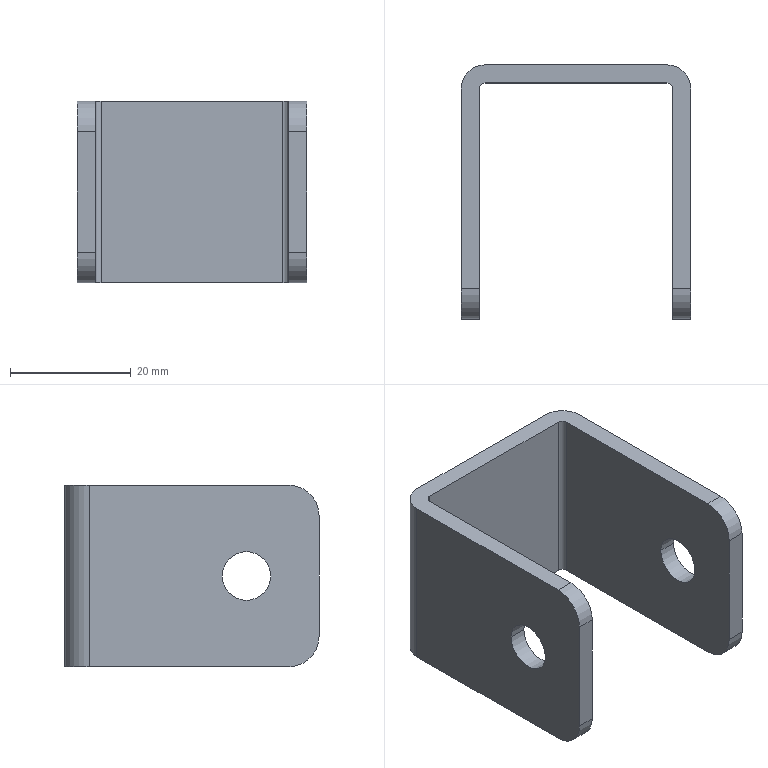Part | NX | features BLEND 1, DATUM_CSYS 1, EXTRACT_DATUM_PLANE 1, EXTRUDE 1, LINKED_BODY 1, SKETCH 1, SUBTRACT 1 | 1 solid | 22 faces | box 38 x 42 x 30 mm | volume 9881 mm3 | cylinder 12 | plane 10 | commonest cylinder face diameters 8 x6 10 x4 2 x2
STEP:
#1=CARTESIAN_POINT('',(-19.,-5.,0.));
#2=VERTEX_POINT('',#1);
#3=CARTESIAN_POINT('',(-19.,-13.,0.));
#4=VERTEX_POINT('',#3);
#5=CARTESIAN_POINT('',(-19.,-9.,0.));
#6=DIRECTION('',(-1.,0.,0.));
#7=DIRECTION('',(0.,0.,1.));
#8=AXIS2_PLACEMENT_3D('',#5,#6,#7);
#9=CIRCLE('',#8,4.);
#10=EDGE_CURVE('',#2,#4,#9,.T.);
#11=ORIENTED_EDGE('',*,*,#10,.F.);
#12=CARTESIAN_POINT('',(-19.,-9.,0.));
#13=DIRECTION('',(-1.,0.,0.));
#14=DIRECTION('',(0.,0.,1.));
#15=AXIS2_PLACEMENT_3D('',#12,#13,#14);
#16=CIRCLE('',#15,4.);
#17=EDGE_CURVE('',#4,#2,#16,.T.);
#18=ORIENTED_EDGE('',*,*,#17,.F.);
#19=EDGE_LOOP('',(#11,#18));
#20=FACE_BOUND('',#19,.T.);
#21=CARTESIAN_POINT('',(-19.,-21.,10.));
#22=VERTEX_POINT('',#21);
#23=CARTESIAN_POINT('',(-19.,-21.,-10.));
#24=VERTEX_POINT('',#23);
#25=CARTESIAN_POINT('',(-19.,-21.,15.));
#26=DIRECTION('',(0.,0.,-1.));
#27=VECTOR('',#26,1000.);
#28=LINE('',#25,#27);
#29=EDGE_CURVE('',#22,#24,#28,.T.);
#30=ORIENTED_EDGE('',*,*,#29,.F.);
#31=CARTESIAN_POINT('',(-19.,-16.,15.));
#32=VERTEX_POINT('',#31);
#33=CARTESIAN_POINT('',(-19.,-16.,10.));
#34=DIRECTION('',(-1.,0.,0.));
#35=DIRECTION('',(0.,0.,1.));
#36=AXIS2_PLACEMENT_3D('',#33,#34,#35);
#37=CIRCLE('',#36,5.);
#38=EDGE_CURVE('',#22,#32,#37,.T.);
#39=ORIENTED_EDGE('',*,*,#38,.T.);
#40=CARTESIAN_POINT('',(-19.,17.,15.));
#41=VERTEX_POINT('',#40);
#42=CARTESIAN_POINT('',(-19.,-21.,15.));
#43=DIRECTION('',(0.,1.,0.));
#44=VECTOR('',#43,1000.);
#45=LINE('',#42,#44);
#46=EDGE_CURVE('',#41,#32,#45,.F.);
#47=ORIENTED_EDGE('',*,*,#46,.F.);
#48=CARTESIAN_POINT('',(-19.,17.,-15.));
#49=VERTEX_POINT('',#48);
#50=CARTESIAN_POINT('',(-19.,17.,15.));
#51=DIRECTION('',(0.,0.,-1.));
#52=VECTOR('',#51,1000.);
#53=LINE('',#50,#52);
#54=EDGE_CURVE('',#41,#49,#53,.T.);
#55=ORIENTED_EDGE('',*,*,#54,.T.);
#56=CARTESIAN_POINT('',(-19.,-16.,-15.));
#57=VERTEX_POINT('',#56);
#58=CARTESIAN_POINT('',(-19.,-16.,-15.));
#59=DIRECTION('',(0.,1.,0.));
#60=VECTOR('',#59,1000.);
#61=LINE('',#58,#60);
#62=EDGE_CURVE('',#57,#49,#61,.T.);
#63=ORIENTED_EDGE('',*,*,#62,.F.);
#64=CARTESIAN_POINT('',(-19.,-16.,-10.));
#65=DIRECTION('',(-1.,0.,0.));
#66=DIRECTION('',(0.,0.,1.));
#67=AXIS2_PLACEMENT_3D('',#64,#65,#66);
#68=CIRCLE('',#67,5.);
#69=EDGE_CURVE('',#57,#24,#68,.T.);
#70=ORIENTED_EDGE('',*,*,#69,.T.);
#71=EDGE_LOOP('',(#30,#39,#47,#55,#63,#70));
#72=FACE_BOUND('',#71,.T.);
#73=CARTESIAN_POINT('',(-19.,-16.,15.));
#74=DIRECTION('',(-1.,0.,0.));
#75=DIRECTION('',(0.,0.,1.));
#76=AXIS2_PLACEMENT_3D('',#73,#74,#75);
#77=PLANE('',#76);
#78=ADVANCED_FACE('',(#20,#72),#77,.T.);
#79=CARTESIAN_POINT('',(-15.,21.,-15.));
#80=VERTEX_POINT('',#79);
#81=CARTESIAN_POINT('',(-15.,17.,-15.));
#82=DIRECTION('',(0.,0.,-1.));
#83=DIRECTION('',(-1.,0.,0.));
#84=AXIS2_PLACEMENT_3D('',#81,#82,#83);
#85=CIRCLE('',#84,4.);
#86=EDGE_CURVE('',#49,#80,#85,.T.);
#87=ORIENTED_EDGE('',*,*,#86,.F.);
#88=ORIENTED_EDGE('',*,*,#54,.F.);
#89=CARTESIAN_POINT('',(-15.,21.,15.));
#90=VERTEX_POINT('',#89);
#91=CARTESIAN_POINT('',(-15.,17.,15.));
#92=DIRECTION('',(0.,0.,-1.));
#93=DIRECTION('',(-1.,0.,0.));
#94=AXIS2_PLACEMENT_3D('',#91,#92,#93);
#95=CIRCLE('',#94,4.);
#96=EDGE_CURVE('',#90,#41,#95,.F.);
#97=ORIENTED_EDGE('',*,*,#96,.F.);
#98=CARTESIAN_POINT('',(-15.,21.,15.));
#99=DIRECTION('',(0.,0.,-1.));
#100=VECTOR('',#99,1000.);
#101=LINE('',#98,#100);
#102=EDGE_CURVE('',#90,#80,#101,.T.);
#103=ORIENTED_EDGE('',*,*,#102,.T.);
#104=EDGE_LOOP('',(#87,#88,#97,#103));
#105=FACE_BOUND('',#104,.T.);
#106=CARTESIAN_POINT('',(-15.,17.,15.));
#107=DIRECTION('',(0.,0.,-1.));
#108=DIRECTION('',(-1.,0.,0.));
#109=AXIS2_PLACEMENT_3D('',#106,#107,#108);
#110=CYLINDRICAL_SURFACE('',#109,4.);
#111=ADVANCED_FACE('',(#105),#110,.T.);
#112=CARTESIAN_POINT('',(15.,21.,-15.));
#113=VERTEX_POINT('',#112);
#114=CARTESIAN_POINT('',(-15.,21.,-15.));
#115=DIRECTION('',(1.,0.,0.));
#116=VECTOR('',#115,1000.);
#117=LINE('',#114,#116);
#118=EDGE_CURVE('',#80,#113,#117,.T.);
#119=ORIENTED_EDGE('',*,*,#118,.F.);
#120=ORIENTED_EDGE('',*,*,#102,.F.);
#121=CARTESIAN_POINT('',(15.,21.,15.));
#122=VERTEX_POINT('',#121);
#123=CARTESIAN_POINT('',(-15.,21.,15.));
#124=DIRECTION('',(1.,0.,0.));
#125=VECTOR('',#124,1000.);
#126=LINE('',#123,#125);
#127=EDGE_CURVE('',#122,#90,#126,.F.);
#128=ORIENTED_EDGE('',*,*,#127,.F.);
#129=CARTESIAN_POINT('',(15.,21.,15.));
#130=DIRECTION('',(0.,0.,-1.));
#131=VECTOR('',#130,1000.);
#132=LINE('',#129,#131);
#133=EDGE_CURVE('',#122,#113,#132,.T.);
#134=ORIENTED_EDGE('',*,*,#133,.T.);
#135=EDGE_LOOP('',(#119,#120,#128,#134));
#136=FACE_BOUND('',#135,.T.);
#137=CARTESIAN_POINT('',(-15.,21.,15.));
#138=DIRECTION('',(0.,1.,0.));
#139=DIRECTION('',(0.,0.,1.));
#140=AXIS2_PLACEMENT_3D('',#137,#138,#139);
#141=PLANE('',#140);
#142=ADVANCED_FACE('',(#136),#141,.T.);
#143=CARTESIAN_POINT('',(19.,17.,-15.));
#144=VERTEX_POINT('',#143);
#145=CARTESIAN_POINT('',(15.,17.,-15.));
#146=DIRECTION('',(0.,0.,-1.));
#147=DIRECTION('',(0.,1.,0.));
#148=AXIS2_PLACEMENT_3D('',#145,#146,#147);
#149=CIRCLE('',#148,4.);
#150=EDGE_CURVE('',#113,#144,#149,.T.);
#151=ORIENTED_EDGE('',*,*,#150,.F.);
#152=ORIENTED_EDGE('',*,*,#133,.F.);
#153=CARTESIAN_POINT('',(19.,17.,15.));
#154=VERTEX_POINT('',#153);
#155=CARTESIAN_POINT('',(15.,17.,15.));
#156=DIRECTION('',(0.,0.,-1.));
#157=DIRECTION('',(0.,1.,0.));
#158=AXIS2_PLACEMENT_3D('',#155,#156,#157);
#159=CIRCLE('',#158,4.);
#160=EDGE_CURVE('',#154,#122,#159,.F.);
#161=ORIENTED_EDGE('',*,*,#160,.F.);
#162=CARTESIAN_POINT('',(19.,17.,15.));
#163=DIRECTION('',(0.,0.,-1.));
#164=VECTOR('',#163,1000.);
#165=LINE('',#162,#164);
#166=EDGE_CURVE('',#154,#144,#165,.T.);
#167=ORIENTED_EDGE('',*,*,#166,.T.);
#168=EDGE_LOOP('',(#151,#152,#161,#167));
#169=FACE_BOUND('',#168,.T.);
#170=CARTESIAN_POINT('',(15.,17.,15.));
#171=DIRECTION('',(0.,0.,-1.));
#172=DIRECTION('',(-1.,0.,0.));
#173=AXIS2_PLACEMENT_3D('',#170,#171,#172);
#174=CYLINDRICAL_SURFACE('',#173,4.);
#175=ADVANCED_FACE('',(#169),#174,.T.);
#176=CARTESIAN_POINT('',(19.,-16.,15.));
#177=VERTEX_POINT('',#176);
#178=CARTESIAN_POINT('',(19.,17.,15.));
#179=DIRECTION('',(0.,-1.,0.));
#180=VECTOR('',#179,1000.);
#181=LINE('',#178,#180);
#182=EDGE_CURVE('',#177,#154,#181,.F.);
#183=ORIENTED_EDGE('',*,*,#182,.F.);
#184=CARTESIAN_POINT('',(19.,-21.,10.));
#185=VERTEX_POINT('',#184);
#186=CARTESIAN_POINT('',(19.,-16.,10.));
#187=DIRECTION('',(1.,0.,0.));
#188=DIRECTION('',(0.,0.,-1.));
#189=AXIS2_PLACEMENT_3D('',#186,#187,#188);
#190=CIRCLE('',#189,5.);
#191=EDGE_CURVE('',#177,#185,#190,.T.);
#192=ORIENTED_EDGE('',*,*,#191,.T.);
#193=CARTESIAN_POINT('',(19.,-21.,-10.));
#194=VERTEX_POINT('',#193);
#195=CARTESIAN_POINT('',(19.,-21.,15.));
#196=DIRECTION('',(0.,0.,-1.));
#197=VECTOR('',#196,1000.);
#198=LINE('',#195,#197);
#199=EDGE_CURVE('',#185,#194,#198,.T.);
#200=ORIENTED_EDGE('',*,*,#199,.T.);
#201=CARTESIAN_POINT('',(19.,-16.,-15.));
#202=VERTEX_POINT('',#201);
#203=CARTESIAN_POINT('',(19.,-16.,-10.));
#204=DIRECTION('',(1.,0.,0.));
#205=DIRECTION('',(0.,0.,-1.));
#206=AXIS2_PLACEMENT_3D('',#203,#204,#205);
#207=CIRCLE('',#206,5.);
#208=EDGE_CURVE('',#194,#202,#207,.T.);
#209=ORIENTED_EDGE('',*,*,#208,.T.);
#210=CARTESIAN_POINT('',(19.,-16.,-15.));
#211=DIRECTION('',(0.,-1.,0.));
#212=VECTOR('',#211,1000.);
#213=LINE('',#210,#212);
#214=EDGE_CURVE('',#144,#202,#213,.T.);
#215=ORIENTED_EDGE('',*,*,#214,.F.);
#216=ORIENTED_EDGE('',*,*,#166,.F.);
#217=EDGE_LOOP('',(#183,#192,#200,#209,#215,#216));
#218=FACE_BOUND('',#217,.T.);
#219=CARTESIAN_POINT('',(19.,-13.,0.));
#220=VERTEX_POINT('',#219);
#221=CARTESIAN_POINT('',(19.,-5.,0.));
#222=VERTEX_POINT('',#221);
#223=CARTESIAN_POINT('',(19.,-9.,0.));
#224=DIRECTION('',(1.,0.,0.));
#225=DIRECTION('',(0.,-1.,0.));
#226=AXIS2_PLACEMENT_3D('',#223,#224,#225);
#227=CIRCLE('',#226,4.);
#228=EDGE_CURVE('',#220,#222,#227,.T.);
#229=ORIENTED_EDGE('',*,*,#228,.F.);
#230=CARTESIAN_POINT('',(19.,-9.,0.));
#231=DIRECTION('',(1.,0.,0.));
#232=DIRECTION('',(0.,1.,0.));
#233=AXIS2_PLACEMENT_3D('',#230,#231,#232);
#234=CIRCLE('',#233,4.);
#235=EDGE_CURVE('',#222,#220,#234,.T.);
#236=ORIENTED_EDGE('',*,*,#235,.F.);
#237=EDGE_LOOP('',(#229,#236));
#238=FACE_BOUND('',#237,.T.);
#239=CARTESIAN_POINT('',(19.,-16.,15.));
#240=DIRECTION('',(1.,0.,0.));
#241=DIRECTION('',(0.,0.,-1.));
#242=AXIS2_PLACEMENT_3D('',#239,#240,#241);
#243=PLANE('',#242);
#244=ADVANCED_FACE('',(#218,#238),#243,.T.);
#245=ORIENTED_EDGE('',*,*,#199,.F.);
#246=CARTESIAN_POINT('',(16.,-21.,10.));
#247=VERTEX_POINT('',#246);
#248=CARTESIAN_POINT('',(16.,-21.,10.));
#249=DIRECTION('',(1.,0.,0.));
#250=VECTOR('',#249,1000.);
#251=LINE('',#248,#250);
#252=EDGE_CURVE('',#185,#247,#251,.F.);
#253=ORIENTED_EDGE('',*,*,#252,.T.);
#254=CARTESIAN_POINT('',(16.,-21.,-10.));
#255=VERTEX_POINT('',#254);
#256=CARTESIAN_POINT('',(16.,-21.,15.));
#257=DIRECTION('',(0.,0.,-1.));
#258=VECTOR('',#257,1000.);
#259=LINE('',#256,#258);
#260=EDGE_CURVE('',#247,#255,#259,.T.);
#261=ORIENTED_EDGE('',*,*,#260,.T.);
#262=CARTESIAN_POINT('',(19.,-21.,-10.));
#263=DIRECTION('',(-1.,0.,0.));
#264=VECTOR('',#263,1000.);
#265=LINE('',#262,#264);
#266=EDGE_CURVE('',#255,#194,#265,.F.);
#267=ORIENTED_EDGE('',*,*,#266,.T.);
#268=EDGE_LOOP('',(#245,#253,#261,#267));
#269=FACE_BOUND('',#268,.T.);
#270=CARTESIAN_POINT('',(19.,-21.,15.));
#271=DIRECTION('',(0.,-1.,0.));
#272=DIRECTION('',(0.,0.,-1.));
#273=AXIS2_PLACEMENT_3D('',#270,#271,#272);
#274=PLANE('',#273);
#275=ADVANCED_FACE('',(#269),#274,.T.);
#276=CARTESIAN_POINT('',(16.,-5.,0.));
#277=VERTEX_POINT('',#276);
#278=CARTESIAN_POINT('',(16.,-13.,0.));
#279=VERTEX_POINT('',#278);
#280=CARTESIAN_POINT('',(16.,-9.,0.));
#281=DIRECTION('',(-1.,0.,0.));
#282=DIRECTION('',(0.,0.,1.));
#283=AXIS2_PLACEMENT_3D('',#280,#281,#282);
#284=CIRCLE('',#283,4.);
#285=EDGE_CURVE('',#277,#279,#284,.T.);
#286=ORIENTED_EDGE('',*,*,#285,.F.);
#287=CARTESIAN_POINT('',(16.,-9.,0.));
#288=DIRECTION('',(-1.,0.,0.));
#289=DIRECTION('',(0.,0.,1.));
#290=AXIS2_PLACEMENT_3D('',#287,#288,#289);
#291=CIRCLE('',#290,4.);
#292=EDGE_CURVE('',#279,#277,#291,.T.);
#293=ORIENTED_EDGE('',*,*,#292,.F.);
#294=EDGE_LOOP('',(#286,#293));
#295=FACE_BOUND('',#294,.T.);
#296=ORIENTED_EDGE('',*,*,#260,.F.);
#297=CARTESIAN_POINT('',(16.,-16.,15.));
#298=VERTEX_POINT('',#297);
#299=CARTESIAN_POINT('',(16.,-16.,10.));
#300=DIRECTION('',(-1.,0.,0.));
#301=DIRECTION('',(0.,0.,1.));
#302=AXIS2_PLACEMENT_3D('',#299,#300,#301);
#303=CIRCLE('',#302,5.);
#304=EDGE_CURVE('',#247,#298,#303,.T.);
#305=ORIENTED_EDGE('',*,*,#304,.T.);
#306=CARTESIAN_POINT('',(16.,17.,15.));
#307=VERTEX_POINT('',#306);
#308=CARTESIAN_POINT('',(16.,-21.,15.));
#309=DIRECTION('',(0.,1.,0.));
#310=VECTOR('',#309,1000.);
#311=LINE('',#308,#310);
#312=EDGE_CURVE('',#307,#298,#311,.F.);
#313=ORIENTED_EDGE('',*,*,#312,.F.);
#314=CARTESIAN_POINT('',(16.,17.,-15.));
#315=VERTEX_POINT('',#314);
#316=CARTESIAN_POINT('',(16.,17.,15.));
#317=DIRECTION('',(0.,0.,-1.));
#318=VECTOR('',#317,1000.);
#319=LINE('',#316,#318);
#320=EDGE_CURVE('',#307,#315,#319,.T.);
#321=ORIENTED_EDGE('',*,*,#320,.T.);
#322=CARTESIAN_POINT('',(16.,-16.,-15.));
#323=VERTEX_POINT('',#322);
#324=CARTESIAN_POINT('',(16.,-16.,-15.));
#325=DIRECTION('',(0.,1.,0.));
#326=VECTOR('',#325,1000.);
#327=LINE('',#324,#326);
#328=EDGE_CURVE('',#323,#315,#327,.T.);
#329=ORIENTED_EDGE('',*,*,#328,.F.);
#330=CARTESIAN_POINT('',(16.,-16.,-10.));
#331=DIRECTION('',(-1.,0.,0.));
#332=DIRECTION('',(0.,0.,1.));
#333=AXIS2_PLACEMENT_3D('',#330,#331,#332);
#334=CIRCLE('',#333,5.);
#335=EDGE_CURVE('',#323,#255,#334,.T.);
#336=ORIENTED_EDGE('',*,*,#335,.T.);
#337=EDGE_LOOP('',(#296,#305,#313,#321,#329,#336));
#338=FACE_BOUND('',#337,.T.);
#339=CARTESIAN_POINT('',(16.,-16.,15.));
#340=DIRECTION('',(-1.,0.,0.));
#341=DIRECTION('',(0.,0.,1.));
#342=AXIS2_PLACEMENT_3D('',#339,#340,#341);
#343=PLANE('',#342);
#344=ADVANCED_FACE('',(#295,#338),#343,.T.);
#345=CARTESIAN_POINT('',(15.,18.,-15.));
#346=VERTEX_POINT('',#345);
#347=CARTESIAN_POINT('',(15.,17.,-15.));
#348=DIRECTION('',(0.,0.,1.));
#349=DIRECTION('',(1.,0.,0.));
#350=AXIS2_PLACEMENT_3D('',#347,#348,#349);
#351=CIRCLE('',#350,1.);
#352=EDGE_CURVE('',#315,#346,#351,.T.);
#353=ORIENTED_EDGE('',*,*,#352,.F.);
#354=ORIENTED_EDGE('',*,*,#320,.F.);
#355=CARTESIAN_POINT('',(15.,18.,15.));
#356=VERTEX_POINT('',#355);
#357=CARTESIAN_POINT('',(15.,17.,15.));
#358=DIRECTION('',(0.,0.,1.));
#359=DIRECTION('',(1.,0.,0.));
#360=AXIS2_PLACEMENT_3D('',#357,#358,#359);
#361=CIRCLE('',#360,1.);
#362=EDGE_CURVE('',#356,#307,#361,.F.);
#363=ORIENTED_EDGE('',*,*,#362,.F.);
#364=CARTESIAN_POINT('',(15.,18.,15.));
#365=DIRECTION('',(0.,0.,-1.));
#366=VECTOR('',#365,1000.);
#367=LINE('',#364,#366);
#368=EDGE_CURVE('',#356,#346,#367,.T.);
#369=ORIENTED_EDGE('',*,*,#368,.T.);
#370=EDGE_LOOP('',(#353,#354,#363,#369));
#371=FACE_BOUND('',#370,.T.);
#372=CARTESIAN_POINT('',(15.,17.,15.));
#373=DIRECTION('',(0.,0.,-1.));
#374=DIRECTION('',(-1.,0.,0.));
#375=AXIS2_PLACEMENT_3D('',#372,#373,#374);
#376=CYLINDRICAL_SURFACE('',#375,1.);
#377=ADVANCED_FACE('',(#371),#376,.F.);
#378=CARTESIAN_POINT('',(-15.,18.,-15.));
#379=VERTEX_POINT('',#378);
#380=CARTESIAN_POINT('',(15.,18.,-15.));
#381=DIRECTION('',(-1.,0.,0.));
#382=VECTOR('',#381,1000.);
#383=LINE('',#380,#382);
#384=EDGE_CURVE('',#346,#379,#383,.T.);
#385=ORIENTED_EDGE('',*,*,#384,.F.);
#386=ORIENTED_EDGE('',*,*,#368,.F.);
#387=CARTESIAN_POINT('',(-15.,18.,15.));
#388=VERTEX_POINT('',#387);
#389=CARTESIAN_POINT('',(15.,18.,15.));
#390=DIRECTION('',(-1.,0.,0.));
#391=VECTOR('',#390,1000.);
#392=LINE('',#389,#391);
#393=EDGE_CURVE('',#388,#356,#392,.F.);
#394=ORIENTED_EDGE('',*,*,#393,.F.);
#395=CARTESIAN_POINT('',(-15.,18.,15.));
#396=DIRECTION('',(0.,0.,-1.));
#397=VECTOR('',#396,1000.);
#398=LINE('',#395,#397);
#399=EDGE_CURVE('',#388,#379,#398,.T.);
#400=ORIENTED_EDGE('',*,*,#399,.T.);
#401=EDGE_LOOP('',(#385,#386,#394,#400));
#402=FACE_BOUND('',#401,.T.);
#403=CARTESIAN_POINT('',(15.,18.,15.));
#404=DIRECTION('',(0.,-1.,0.));
#405=DIRECTION('',(0.,0.,-1.));
#406=AXIS2_PLACEMENT_3D('',#403,#404,#405);
#407=PLANE('',#406);
#408=ADVANCED_FACE('',(#402),#407,.T.);
#409=CARTESIAN_POINT('',(-16.,17.,-15.));
#410=VERTEX_POINT('',#409);
#411=CARTESIAN_POINT('',(-15.,17.,-15.));
#412=DIRECTION('',(0.,0.,1.));
#413=DIRECTION('',(0.,1.,0.));
#414=AXIS2_PLACEMENT_3D('',#411,#412,#413);
#415=CIRCLE('',#414,1.);
#416=EDGE_CURVE('',#379,#410,#415,.T.);
#417=ORIENTED_EDGE('',*,*,#416,.F.);
#418=ORIENTED_EDGE('',*,*,#399,.F.);
#419=CARTESIAN_POINT('',(-16.,17.,15.));
#420=VERTEX_POINT('',#419);
#421=CARTESIAN_POINT('',(-15.,17.,15.));
#422=DIRECTION('',(0.,0.,1.));
#423=DIRECTION('',(0.,1.,0.));
#424=AXIS2_PLACEMENT_3D('',#421,#422,#423);
#425=CIRCLE('',#424,1.);
#426=EDGE_CURVE('',#420,#388,#425,.F.);
#427=ORIENTED_EDGE('',*,*,#426,.F.);
#428=CARTESIAN_POINT('',(-16.,17.,15.));
#429=DIRECTION('',(0.,0.,-1.));
#430=VECTOR('',#429,1000.);
#431=LINE('',#428,#430);
#432=EDGE_CURVE('',#420,#410,#431,.T.);
#433=ORIENTED_EDGE('',*,*,#432,.T.);
#434=EDGE_LOOP('',(#417,#418,#427,#433));
#435=FACE_BOUND('',#434,.T.);
#436=CARTESIAN_POINT('',(-15.,17.,15.));
#437=DIRECTION('',(0.,0.,-1.));
#438=DIRECTION('',(-1.,0.,0.));
#439=AXIS2_PLACEMENT_3D('',#436,#437,#438);
#440=CYLINDRICAL_SURFACE('',#439,1.);
#441=ADVANCED_FACE('',(#435),#440,.F.);
#442=CARTESIAN_POINT('',(-16.,-13.,0.));
#443=VERTEX_POINT('',#442);
#444=CARTESIAN_POINT('',(-16.,-5.,0.));
#445=VERTEX_POINT('',#444);
#446=CARTESIAN_POINT('',(-16.,-9.,0.));
#447=DIRECTION('',(1.,0.,0.));
#448=DIRECTION('',(0.,0.,-1.));
#449=AXIS2_PLACEMENT_3D('',#446,#447,#448);
#450=CIRCLE('',#449,4.);
#451=EDGE_CURVE('',#443,#445,#450,.T.);
#452=ORIENTED_EDGE('',*,*,#451,.F.);
#453=CARTESIAN_POINT('',(-16.,-9.,0.));
#454=DIRECTION('',(1.,0.,0.));
#455=DIRECTION('',(0.,0.,-1.));
#456=AXIS2_PLACEMENT_3D('',#453,#454,#455);
#457=CIRCLE('',#456,4.);
#458=EDGE_CURVE('',#445,#443,#457,.T.);
#459=ORIENTED_EDGE('',*,*,#458,.F.);
#460=EDGE_LOOP('',(#452,#459));
#461=FACE_BOUND('',#460,.T.);
#462=CARTESIAN_POINT('',(-16.,-16.,15.));
#463=VERTEX_POINT('',#462);
#464=CARTESIAN_POINT('',(-16.,17.,15.));
#465=DIRECTION('',(0.,-1.,0.));
#466=VECTOR('',#465,1000.);
#467=LINE('',#464,#466);
#468=EDGE_CURVE('',#463,#420,#467,.F.);
#469=ORIENTED_EDGE('',*,*,#468,.F.);
#470=CARTESIAN_POINT('',(-16.,-21.,10.));
#471=VERTEX_POINT('',#470);
#472=CARTESIAN_POINT('',(-16.,-16.,10.));
#473=DIRECTION('',(1.,0.,0.));
#474=DIRECTION('',(0.,0.,-1.));
#475=AXIS2_PLACEMENT_3D('',#472,#473,#474);
#476=CIRCLE('',#475,5.);
#477=EDGE_CURVE('',#463,#471,#476,.T.);
#478=ORIENTED_EDGE('',*,*,#477,.T.);
#479=CARTESIAN_POINT('',(-16.,-21.,-10.));
#480=VERTEX_POINT('',#479);
#481=CARTESIAN_POINT('',(-16.,-21.,15.));
#482=DIRECTION('',(0.,0.,-1.));
#483=VECTOR('',#482,1000.);
#484=LINE('',#481,#483);
#485=EDGE_CURVE('',#471,#480,#484,.T.);
#486=ORIENTED_EDGE('',*,*,#485,.T.);
#487=CARTESIAN_POINT('',(-16.,-16.,-15.));
#488=VERTEX_POINT('',#487);
#489=CARTESIAN_POINT('',(-16.,-16.,-10.));
#490=DIRECTION('',(1.,0.,0.));
#491=DIRECTION('',(0.,0.,-1.));
#492=AXIS2_PLACEMENT_3D('',#489,#490,#491);
#493=CIRCLE('',#492,5.);
#494=EDGE_CURVE('',#480,#488,#493,.T.);
#495=ORIENTED_EDGE('',*,*,#494,.T.);
#496=CARTESIAN_POINT('',(-16.,-16.,-15.));
#497=DIRECTION('',(0.,-1.,0.));
#498=VECTOR('',#497,1000.);
#499=LINE('',#496,#498);
#500=EDGE_CURVE('',#410,#488,#499,.T.);
#501=ORIENTED_EDGE('',*,*,#500,.F.);
#502=ORIENTED_EDGE('',*,*,#432,.F.);
#503=EDGE_LOOP('',(#469,#478,#486,#495,#501,#502));
#504=FACE_BOUND('',#503,.T.);
#505=CARTESIAN_POINT('',(-16.,-16.,15.));
#506=DIRECTION('',(1.,0.,0.));
#507=DIRECTION('',(0.,0.,-1.));
#508=AXIS2_PLACEMENT_3D('',#505,#506,#507);
#509=PLANE('',#508);
#510=ADVANCED_FACE('',(#461,#504),#509,.T.);
#511=ORIENTED_EDGE('',*,*,#485,.F.);
#512=CARTESIAN_POINT('',(-19.,-21.,10.));
#513=DIRECTION('',(1.,0.,0.));
#514=VECTOR('',#513,1000.);
#515=LINE('',#512,#514);
#516=EDGE_CURVE('',#471,#22,#515,.F.);
#517=ORIENTED_EDGE('',*,*,#516,.T.);
#518=ORIENTED_EDGE('',*,*,#29,.T.);
#519=CARTESIAN_POINT('',(-16.,-21.,-10.));
#520=DIRECTION('',(-1.,0.,0.));
#521=VECTOR('',#520,1000.);
#522=LINE('',#519,#521);
#523=EDGE_CURVE('',#24,#480,#522,.F.);
#524=ORIENTED_EDGE('',*,*,#523,.T.);
#525=EDGE_LOOP('',(#511,#517,#518,#524));
#526=FACE_BOUND('',#525,.T.);
#527=CARTESIAN_POINT('',(-16.,-21.,15.));
#528=DIRECTION('',(0.,-1.,0.));
#529=DIRECTION('',(0.,0.,-1.));
#530=AXIS2_PLACEMENT_3D('',#527,#528,#529);
#531=PLANE('',#530);
#532=ADVANCED_FACE('',(#526),#531,.T.);
#533=ORIENTED_EDGE('',*,*,#46,.T.);
#534=CARTESIAN_POINT('',(-16.,-16.,15.));
#535=DIRECTION('',(1.,0.,0.));
#536=VECTOR('',#535,1000.);
#537=LINE('',#534,#536);
#538=EDGE_CURVE('',#32,#463,#537,.T.);
#539=ORIENTED_EDGE('',*,*,#538,.T.);
#540=ORIENTED_EDGE('',*,*,#468,.T.);
#541=ORIENTED_EDGE('',*,*,#426,.T.);
#542=ORIENTED_EDGE('',*,*,#393,.T.);
#543=ORIENTED_EDGE('',*,*,#362,.T.);
#544=ORIENTED_EDGE('',*,*,#312,.T.);
#545=CARTESIAN_POINT('',(19.,-16.,15.));
#546=DIRECTION('',(1.,0.,0.));
#547=VECTOR('',#546,1000.);
#548=LINE('',#545,#547);
#549=EDGE_CURVE('',#298,#177,#548,.T.);
#550=ORIENTED_EDGE('',*,*,#549,.T.);
#551=ORIENTED_EDGE('',*,*,#182,.T.);
#552=ORIENTED_EDGE('',*,*,#160,.T.);
#553=ORIENTED_EDGE('',*,*,#127,.T.);
#554=ORIENTED_EDGE('',*,*,#96,.T.);
#555=EDGE_LOOP('',(#533,#539,#540,#541,#542,#543,#544,#550,#551,#552,#553,#554));
#556=FACE_BOUND('',#555,.T.);
#557=CARTESIAN_POINT('',(-15.,17.,15.));
#558=DIRECTION('',(0.,0.,-1.));
#559=DIRECTION('',(-1.,0.,0.));
#560=AXIS2_PLACEMENT_3D('',#557,#558,#559);
#561=PLANE('',#560);
#562=ADVANCED_FACE('',(#556),#561,.F.);
#563=ORIENTED_EDGE('',*,*,#214,.T.);
#564=CARTESIAN_POINT('',(-15.,-16.,-15.));
#565=DIRECTION('',(-1.,0.,0.));
#566=VECTOR('',#565,1000.);
#567=LINE('',#564,#566);
#568=EDGE_CURVE('',#202,#323,#567,.T.);
#569=ORIENTED_EDGE('',*,*,#568,.T.);
#570=ORIENTED_EDGE('',*,*,#328,.T.);
#571=ORIENTED_EDGE('',*,*,#352,.T.);
#572=ORIENTED_EDGE('',*,*,#384,.T.);
#573=ORIENTED_EDGE('',*,*,#416,.T.);
#574=ORIENTED_EDGE('',*,*,#500,.T.);
#575=CARTESIAN_POINT('',(-15.,-16.,-15.));
#576=DIRECTION('',(-1.,0.,0.));
#577=VECTOR('',#576,1000.);
#578=LINE('',#575,#577);
#579=EDGE_CURVE('',#488,#57,#578,.T.);
#580=ORIENTED_EDGE('',*,*,#579,.T.);
#581=ORIENTED_EDGE('',*,*,#62,.T.);
#582=ORIENTED_EDGE('',*,*,#86,.T.);
#583=ORIENTED_EDGE('',*,*,#118,.T.);
#584=ORIENTED_EDGE('',*,*,#150,.T.);
#585=EDGE_LOOP('',(#563,#569,#570,#571,#572,#573,#574,#580,#581,#582,#583,#584));
#586=FACE_BOUND('',#585,.T.);
#587=CARTESIAN_POINT('',(-15.,17.,-15.));
#588=DIRECTION('',(0.,0.,-1.));
#589=DIRECTION('',(-1.,0.,0.));
#590=AXIS2_PLACEMENT_3D('',#587,#588,#589);
#591=PLANE('',#590);
#592=ADVANCED_FACE('',(#586),#591,.T.);
#593=ORIENTED_EDGE('',*,*,#38,.F.);
#594=ORIENTED_EDGE('',*,*,#516,.F.);
#595=ORIENTED_EDGE('',*,*,#477,.F.);
#596=ORIENTED_EDGE('',*,*,#538,.F.);
#597=EDGE_LOOP('',(#593,#594,#595,#596));
#598=FACE_BOUND('',#597,.T.);
#599=CARTESIAN_POINT('',(-15.,-16.,10.));
#600=DIRECTION('',(-1.,0.,0.));
#601=DIRECTION('',(0.,0.,1.));
#602=AXIS2_PLACEMENT_3D('',#599,#600,#601);
#603=CYLINDRICAL_SURFACE('',#602,5.);
#604=ADVANCED_FACE('',(#598),#603,.T.);
#605=ORIENTED_EDGE('',*,*,#304,.F.);
#606=ORIENTED_EDGE('',*,*,#252,.F.);
#607=ORIENTED_EDGE('',*,*,#191,.F.);
#608=ORIENTED_EDGE('',*,*,#549,.F.);
#609=EDGE_LOOP('',(#605,#606,#607,#608));
#610=FACE_BOUND('',#609,.T.);
#611=CARTESIAN_POINT('',(-15.,-16.,10.));
#612=DIRECTION('',(-1.,0.,0.));
#613=DIRECTION('',(0.,0.,1.));
#614=AXIS2_PLACEMENT_3D('',#611,#612,#613);
#615=CYLINDRICAL_SURFACE('',#614,5.);
#616=ADVANCED_FACE('',(#610),#615,.T.);
#617=ORIENTED_EDGE('',*,*,#208,.F.);
#618=ORIENTED_EDGE('',*,*,#266,.F.);
#619=ORIENTED_EDGE('',*,*,#335,.F.);
#620=ORIENTED_EDGE('',*,*,#568,.F.);
#621=EDGE_LOOP('',(#617,#618,#619,#620));
#622=FACE_BOUND('',#621,.T.);
#623=CARTESIAN_POINT('',(-15.,-16.,-10.));
#624=DIRECTION('',(-1.,0.,0.));
#625=DIRECTION('',(0.,0.,1.));
#626=AXIS2_PLACEMENT_3D('',#623,#624,#625);
#627=CYLINDRICAL_SURFACE('',#626,5.);
#628=ADVANCED_FACE('',(#622),#627,.T.);
#629=ORIENTED_EDGE('',*,*,#494,.F.);
#630=ORIENTED_EDGE('',*,*,#523,.F.);
#631=ORIENTED_EDGE('',*,*,#69,.F.);
#632=ORIENTED_EDGE('',*,*,#579,.F.);
#633=EDGE_LOOP('',(#629,#630,#631,#632));
#634=FACE_BOUND('',#633,.T.);
#635=CARTESIAN_POINT('',(-15.,-16.,-10.));
#636=DIRECTION('',(-1.,0.,0.));
#637=DIRECTION('',(0.,0.,1.));
#638=AXIS2_PLACEMENT_3D('',#635,#636,#637);
#639=CYLINDRICAL_SURFACE('',#638,5.);
#640=ADVANCED_FACE('',(#634),#639,.T.);
#641=ORIENTED_EDGE('',*,*,#17,.T.);
#642=CARTESIAN_POINT('',(-25.,-5.,0.));
#643=DIRECTION('',(1.,0.,0.));
#644=VECTOR('',#643,1000.);
#645=LINE('',#642,#644);
#646=EDGE_CURVE('',#445,#2,#645,.F.);
#647=ORIENTED_EDGE('',*,*,#646,.F.);
#648=ORIENTED_EDGE('',*,*,#458,.T.);
#649=CARTESIAN_POINT('',(-25.,-13.,0.));
#650=DIRECTION('',(1.,0.,0.));
#651=VECTOR('',#650,1000.);
#652=LINE('',#649,#651);
#653=EDGE_CURVE('',#4,#443,#652,.T.);
#654=ORIENTED_EDGE('',*,*,#653,.F.);
#655=EDGE_LOOP('',(#641,#647,#648,#654));
#656=FACE_BOUND('',#655,.T.);
#657=CARTESIAN_POINT('',(19.,-9.,0.));
#658=DIRECTION('',(-1.,0.,0.));
#659=DIRECTION('',(0.,-1.,0.));
#660=AXIS2_PLACEMENT_3D('',#657,#658,#659);
#661=CYLINDRICAL_SURFACE('',#660,4.);
#662=ADVANCED_FACE('',(#656),#661,.F.);
#663=ORIENTED_EDGE('',*,*,#10,.T.);
#664=ORIENTED_EDGE('',*,*,#653,.T.);
#665=ORIENTED_EDGE('',*,*,#451,.T.);
#666=ORIENTED_EDGE('',*,*,#646,.T.);
#667=EDGE_LOOP('',(#663,#664,#665,#666));
#668=FACE_BOUND('',#667,.T.);
#669=CARTESIAN_POINT('',(19.,-9.,0.));
#670=DIRECTION('',(-1.,0.,0.));
#671=DIRECTION('',(0.,-1.,0.));
#672=AXIS2_PLACEMENT_3D('',#669,#670,#671);
#673=CYLINDRICAL_SURFACE('',#672,4.);
#674=ADVANCED_FACE('',(#668),#673,.F.);
#675=ORIENTED_EDGE('',*,*,#285,.T.);
#676=CARTESIAN_POINT('',(-25.,-13.,0.));
#677=DIRECTION('',(1.,0.,0.));
#678=VECTOR('',#677,1000.);
#679=LINE('',#676,#678);
#680=EDGE_CURVE('',#279,#220,#679,.T.);
#681=ORIENTED_EDGE('',*,*,#680,.T.);
#682=ORIENTED_EDGE('',*,*,#228,.T.);
#683=CARTESIAN_POINT('',(-25.,-5.,0.));
#684=DIRECTION('',(1.,0.,0.));
#685=VECTOR('',#684,1000.);
#686=LINE('',#683,#685);
#687=EDGE_CURVE('',#222,#277,#686,.F.);
#688=ORIENTED_EDGE('',*,*,#687,.T.);
#689=EDGE_LOOP('',(#675,#681,#682,#688));
#690=FACE_BOUND('',#689,.T.);
#691=CARTESIAN_POINT('',(19.,-9.,0.));
#692=DIRECTION('',(-1.,0.,0.));
#693=DIRECTION('',(0.,-1.,0.));
#694=AXIS2_PLACEMENT_3D('',#691,#692,#693);
#695=CYLINDRICAL_SURFACE('',#694,4.);
#696=ADVANCED_FACE('',(#690),#695,.F.);
#697=ORIENTED_EDGE('',*,*,#292,.T.);
#698=ORIENTED_EDGE('',*,*,#687,.F.);
#699=ORIENTED_EDGE('',*,*,#235,.T.);
#700=ORIENTED_EDGE('',*,*,#680,.F.);
#701=EDGE_LOOP('',(#697,#698,#699,#700));
#702=FACE_BOUND('',#701,.T.);
#703=CARTESIAN_POINT('',(19.,-9.,0.));
#704=DIRECTION('',(-1.,0.,0.));
#705=DIRECTION('',(0.,-1.,0.));
#706=AXIS2_PLACEMENT_3D('',#703,#704,#705);
#707=CYLINDRICAL_SURFACE('',#706,4.);
#708=ADVANCED_FACE('',(#702),#707,.F.);
#709=CLOSED_SHELL('',(#78,#111,#142,#175,#244,#275,#344,#377,#408,#441,#510,#532,#562,#592,#604,#616,#628,#640,#662,#674,#696,#708));
#710=MANIFOLD_SOLID_BREP('',#709);
#711=(LENGTH_UNIT()NAMED_UNIT(*)SI_UNIT(.MILLI.,.METRE.));
#712=UNCERTAINTY_MEASURE_WITH_UNIT(LENGTH_MEASURE(0.00001),#711,'','');
#713=(NAMED_UNIT(*)PLANE_ANGLE_UNIT()SI_UNIT($,.RADIAN.));
#714=(NAMED_UNIT(*)SI_UNIT($,.STERADIAN.)SOLID_ANGLE_UNIT());
#715=(GEOMETRIC_REPRESENTATION_CONTEXT(3)GLOBAL_UNCERTAINTY_ASSIGNED_CONTEXT((#712))GLOBAL_UNIT_ASSIGNED_CONTEXT((#711,#713,#714))REPRESENTATION_CONTEXT('',''));
#716=ADVANCED_BREP_SHAPE_REPRESENTATION('',(#710),#715);